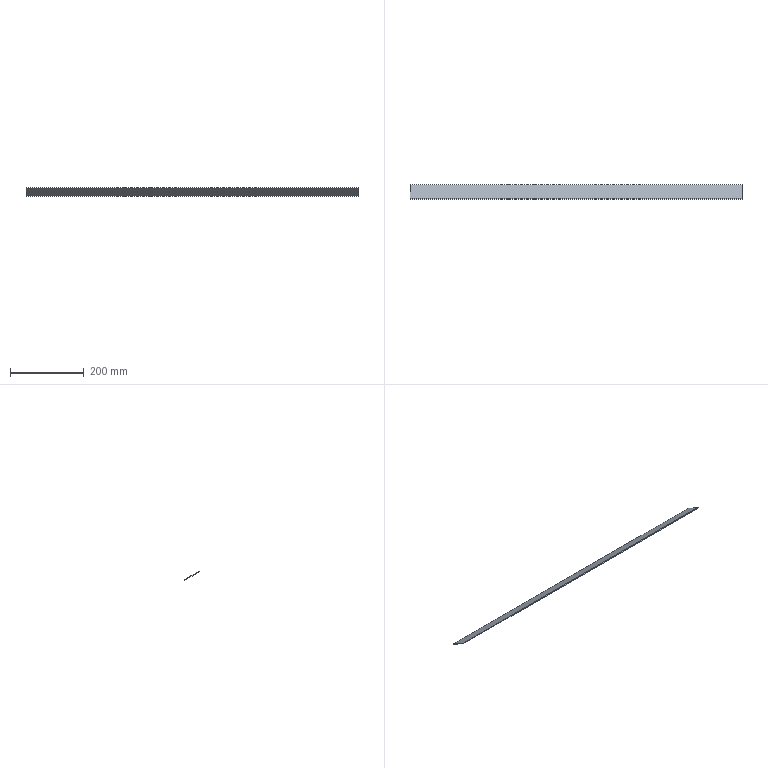Part | SolidWorks | features BaseBody 1 | 1 solid | 6 faces | box 898 x 40 x 23.094 mm | volume 59882 mm3 | plane 6
STEP:
#1=CARTESIAN_POINT('',(898.,40.,1.732));
#2=VERTEX_POINT('',#1);
#3=CARTESIAN_POINT('',(898.,40.,0.));
#4=VERTEX_POINT('',#3);
#5=CARTESIAN_POINT('',(898.,40.,0.));
#6=DIRECTION('',(0.,0.,-1.));
#7=VECTOR('',#6,1000.);
#8=LINE('',#5,#7);
#9=EDGE_CURVE('',#2,#4,#8,.T.);
#10=ORIENTED_EDGE('',*,*,#9,.T.);
#11=CARTESIAN_POINT('',(0.,40.,0.));
#12=VERTEX_POINT('',#11);
#13=CARTESIAN_POINT('',(898.,40.,0.));
#14=DIRECTION('',(-1.,0.,0.));
#15=VECTOR('',#14,1000.);
#16=LINE('',#13,#15);
#17=EDGE_CURVE('',#4,#12,#16,.T.);
#18=ORIENTED_EDGE('',*,*,#17,.T.);
#19=CARTESIAN_POINT('',(0.,40.,1.732));
#20=VERTEX_POINT('',#19);
#21=CARTESIAN_POINT('',(0.,40.,0.));
#22=DIRECTION('',(0.,0.,1.));
#23=VECTOR('',#22,1000.);
#24=LINE('',#21,#23);
#25=EDGE_CURVE('',#12,#20,#24,.T.);
#26=ORIENTED_EDGE('',*,*,#25,.T.);
#27=CARTESIAN_POINT('',(898.,40.,1.732));
#28=DIRECTION('',(-1.,0.,0.));
#29=VECTOR('',#28,1000.);
#30=LINE('',#27,#29);
#31=EDGE_CURVE('',#2,#20,#30,.T.);
#32=ORIENTED_EDGE('',*,*,#31,.F.);
#33=EDGE_LOOP('',(#10,#18,#26,#32));
#34=FACE_OUTER_BOUND('',#33,.T.);
#35=CARTESIAN_POINT('',(0.,40.,0.));
#36=DIRECTION('',(0.,-1.,0.));
#37=DIRECTION('',(0.,0.,-1.));
#38=AXIS2_PLACEMENT_3D('',#35,#36,#37);
#39=PLANE('',#38);
#40=ADVANCED_FACE('',(#34),#39,.F.);
#41=CARTESIAN_POINT('',(0.,0.,23.094));
#42=VERTEX_POINT('',#41);
#43=CARTESIAN_POINT('',(0.,3.,23.094));
#44=VERTEX_POINT('',#43);
#45=CARTESIAN_POINT('',(0.,0.,23.094));
#46=DIRECTION('',(0.,1.,0.));
#47=VECTOR('',#46,1000.);
#48=LINE('',#45,#47);
#49=EDGE_CURVE('',#42,#44,#48,.T.);
#50=ORIENTED_EDGE('',*,*,#49,.F.);
#51=CARTESIAN_POINT('',(898.,0.,23.094));
#52=VERTEX_POINT('',#51);
#53=CARTESIAN_POINT('',(898.,0.,23.094));
#54=DIRECTION('',(-1.,0.,0.));
#55=VECTOR('',#54,1000.);
#56=LINE('',#53,#55);
#57=EDGE_CURVE('',#52,#42,#56,.T.);
#58=ORIENTED_EDGE('',*,*,#57,.F.);
#59=CARTESIAN_POINT('',(898.,3.,23.094));
#60=VERTEX_POINT('',#59);
#61=CARTESIAN_POINT('',(898.,0.,23.094));
#62=DIRECTION('',(0.,1.,0.));
#63=VECTOR('',#62,1000.);
#64=LINE('',#61,#63);
#65=EDGE_CURVE('',#52,#60,#64,.T.);
#66=ORIENTED_EDGE('',*,*,#65,.T.);
#67=CARTESIAN_POINT('',(898.,3.,23.094));
#68=DIRECTION('',(1.,0.,0.));
#69=VECTOR('',#68,1000.);
#70=LINE('',#67,#69);
#71=EDGE_CURVE('',#44,#60,#70,.T.);
#72=ORIENTED_EDGE('',*,*,#71,.F.);
#73=EDGE_LOOP('',(#50,#58,#66,#72));
#74=FACE_OUTER_BOUND('',#73,.T.);
#75=CARTESIAN_POINT('',(0.,0.,23.094));
#76=DIRECTION('',(0.,0.,-1.));
#77=DIRECTION('',(0.,-1.,0.));
#78=AXIS2_PLACEMENT_3D('',#75,#76,#77);
#79=PLANE('',#78);
#80=ADVANCED_FACE('',(#74),#79,.F.);
#81=ORIENTED_EDGE('',*,*,#25,.F.);
#82=CARTESIAN_POINT('',(0.,40.,0.));
#83=DIRECTION('',(0.,-0.866,0.5));
#84=VECTOR('',#83,1000.);
#85=LINE('',#82,#84);
#86=EDGE_CURVE('',#12,#42,#85,.T.);
#87=ORIENTED_EDGE('',*,*,#86,.T.);
#88=ORIENTED_EDGE('',*,*,#49,.T.);
#89=CARTESIAN_POINT('',(0.,40.75,1.299));
#90=DIRECTION('',(0.,-0.866,0.5));
#91=VECTOR('',#90,1000.);
#92=LINE('',#89,#91);
#93=EDGE_CURVE('',#20,#44,#92,.T.);
#94=ORIENTED_EDGE('',*,*,#93,.F.);
#95=EDGE_LOOP('',(#81,#87,#88,#94));
#96=FACE_OUTER_BOUND('',#95,.T.);
#97=CARTESIAN_POINT('',(0.,0.,0.));
#98=DIRECTION('',(-1.,0.,0.));
#99=DIRECTION('',(0.,0.,1.));
#100=AXIS2_PLACEMENT_3D('',#97,#98,#99);
#101=PLANE('',#100);
#102=ADVANCED_FACE('',(#96),#101,.T.);
#103=CARTESIAN_POINT('',(898.,40.,0.));
#104=DIRECTION('',(0.,-0.866,0.5));
#105=VECTOR('',#104,1000.);
#106=LINE('',#103,#105);
#107=EDGE_CURVE('',#4,#52,#106,.T.);
#108=ORIENTED_EDGE('',*,*,#107,.F.);
#109=ORIENTED_EDGE('',*,*,#9,.F.);
#110=CARTESIAN_POINT('',(898.,40.75,1.299));
#111=DIRECTION('',(0.,-0.866,0.5));
#112=VECTOR('',#111,1000.);
#113=LINE('',#110,#112);
#114=EDGE_CURVE('',#2,#60,#113,.T.);
#115=ORIENTED_EDGE('',*,*,#114,.T.);
#116=ORIENTED_EDGE('',*,*,#65,.F.);
#117=EDGE_LOOP('',(#108,#109,#115,#116));
#118=FACE_OUTER_BOUND('',#117,.T.);
#119=CARTESIAN_POINT('',(898.,0.,0.));
#120=DIRECTION('',(-1.,0.,0.));
#121=DIRECTION('',(0.,0.,1.));
#122=AXIS2_PLACEMENT_3D('',#119,#120,#121);
#123=PLANE('',#122);
#124=ADVANCED_FACE('',(#118),#123,.F.);
#125=ORIENTED_EDGE('',*,*,#86,.F.);
#126=ORIENTED_EDGE('',*,*,#17,.F.);
#127=ORIENTED_EDGE('',*,*,#107,.T.);
#128=ORIENTED_EDGE('',*,*,#57,.T.);
#129=EDGE_LOOP('',(#125,#126,#127,#128));
#130=FACE_OUTER_BOUND('',#129,.T.);
#131=CARTESIAN_POINT('',(898.,40.,0.));
#132=DIRECTION('',(0.,-0.5,-0.866));
#133=DIRECTION('',(0.,-0.866,0.5));
#134=AXIS2_PLACEMENT_3D('',#131,#132,#133);
#135=PLANE('',#134);
#136=ADVANCED_FACE('',(#130),#135,.T.);
#137=ORIENTED_EDGE('',*,*,#114,.F.);
#138=ORIENTED_EDGE('',*,*,#31,.T.);
#139=ORIENTED_EDGE('',*,*,#93,.T.);
#140=ORIENTED_EDGE('',*,*,#71,.T.);
#141=EDGE_LOOP('',(#137,#138,#139,#140));
#142=FACE_OUTER_BOUND('',#141,.T.);
#143=CARTESIAN_POINT('',(898.,40.75,1.299));
#144=DIRECTION('',(0.,-0.5,-0.866));
#145=DIRECTION('',(0.,-0.866,0.5));
#146=AXIS2_PLACEMENT_3D('',#143,#144,#145);
#147=PLANE('',#146);
#148=ADVANCED_FACE('',(#142),#147,.F.);
#149=CLOSED_SHELL('',(#40,#80,#102,#124,#136,#148));
#150=MANIFOLD_SOLID_BREP('',#149);
#151=CARTESIAN_POINT('',(0.,0.,0.));
#152=DIRECTION('',(0.,0.,1.));
#153=DIRECTION('',(1.,0.,0.));
#154=AXIS2_PLACEMENT_3D('',#151,#152,#153);
#155=(LENGTH_UNIT()NAMED_UNIT(*)SI_UNIT(.MILLI.,.METRE.));
#156=UNCERTAINTY_MEASURE_WITH_UNIT(LENGTH_MEASURE(0.00001),#155,'','');
#157=(NAMED_UNIT(*)PLANE_ANGLE_UNIT()SI_UNIT($,.RADIAN.));
#158=(NAMED_UNIT(*)SI_UNIT($,.STERADIAN.)SOLID_ANGLE_UNIT());
#159=(GEOMETRIC_REPRESENTATION_CONTEXT(3)GLOBAL_UNCERTAINTY_ASSIGNED_CONTEXT((#156))GLOBAL_UNIT_ASSIGNED_CONTEXT((#155,#157,#158))REPRESENTATION_CONTEXT('',''));
#160=ADVANCED_BREP_SHAPE_REPRESENTATION('',(#150,#154),#159);